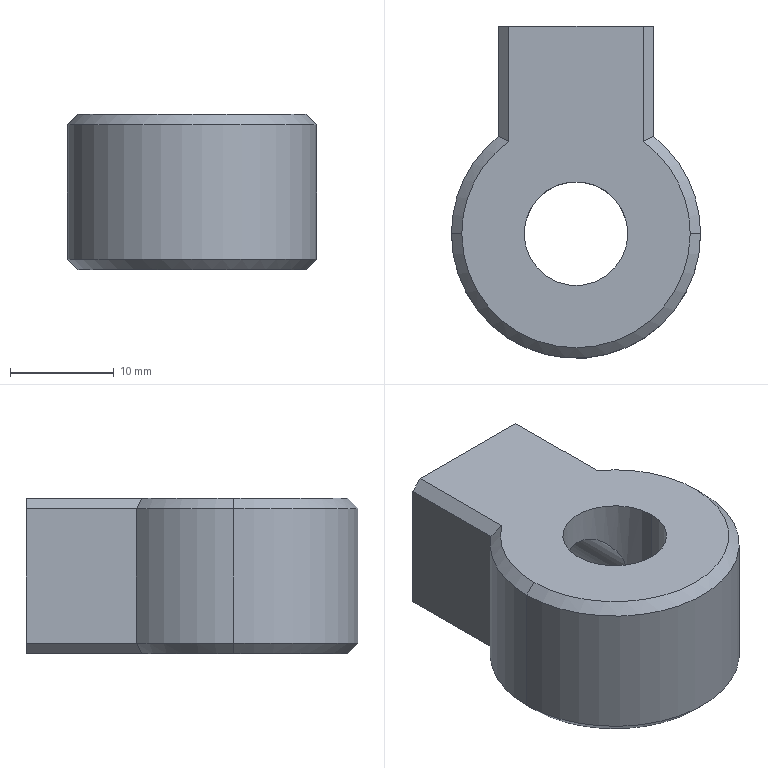Part | SolidWorks | features HoleWzd 2, Chamfer 1, Extrusion 1 | 1 solid | 22 faces | box 24 x 32 x 15 mm | volume 6636 mm3 | plane 9 | cylinder 7 | cone 6 | commonest cylinder face diameters 24 x3 8.5 x2 10 x2
STEP:
#1=CARTESIAN_POINT('',(11.,0.,7.5));
#2=VERTEX_POINT('',#1);
#3=CARTESIAN_POINT('',(6.5,8.874,7.5));
#4=VERTEX_POINT('',#3);
#5=CARTESIAN_POINT('',(0.,0.,7.5));
#6=DIRECTION('',(0.,0.,1.));
#7=DIRECTION('',(1.,0.,0.));
#8=AXIS2_PLACEMENT_3D('',#5,#6,#7);
#9=CIRCLE('',#8,11.);
#10=EDGE_CURVE('',#2,#4,#9,.T.);
#11=ORIENTED_EDGE('',*,*,#10,.F.);
#12=CARTESIAN_POINT('',(12.,0.,6.5));
#13=VERTEX_POINT('',#12);
#14=CARTESIAN_POINT('',(11.,0.,7.5));
#15=DIRECTION('',(0.7071,0.,-0.7071));
#16=VECTOR('',#15,1000.);
#17=LINE('',#14,#16);
#18=EDGE_CURVE('',#2,#13,#17,.T.);
#19=ORIENTED_EDGE('',*,*,#18,.T.);
#20=CARTESIAN_POINT('',(7.5,9.367,6.5));
#21=VERTEX_POINT('',#20);
#22=CARTESIAN_POINT('',(0.,0.,6.5));
#23=DIRECTION('',(0.,0.,-1.));
#24=DIRECTION('',(1.,0.,0.));
#25=AXIS2_PLACEMENT_3D('',#22,#23,#24);
#26=CIRCLE('',#25,12.);
#27=EDGE_CURVE('',#21,#13,#26,.T.);
#28=ORIENTED_EDGE('',*,*,#27,.F.);
#29=CARTESIAN_POINT('',(6.5,8.874,7.5));
#30=CARTESIAN_POINT('',(6.832,9.043,7.168));
#31=CARTESIAN_POINT('',(7.166,9.207,6.834));
#32=CARTESIAN_POINT('',(7.5,9.367,6.5));
#33=B_SPLINE_CURVE_WITH_KNOTS('',3,(#29,#30,#31,#32),.UNSPECIFIED.,.F.,.F.,(4,4),(0.,0.001498),.UNSPECIFIED.);
#34=EDGE_CURVE('',#4,#21,#33,.T.);
#35=ORIENTED_EDGE('',*,*,#34,.F.);
#36=EDGE_LOOP('',(#11,#19,#28,#35));
#37=FACE_OUTER_BOUND('',#36,.T.);
#38=CARTESIAN_POINT('',(0.,0.,7.5));
#39=DIRECTION('',(0.,0.,-1.));
#40=DIRECTION('',(-1.,0.,0.));
#41=AXIS2_PLACEMENT_3D('',#38,#39,#40);
#42=CONICAL_SURFACE('',#41,11.,0.7854);
#43=ADVANCED_FACE('',(#37),#42,.T.);
#44=ORIENTED_EDGE('',*,*,#18,.F.);
#45=CARTESIAN_POINT('',(-11.,0.,7.5));
#46=VERTEX_POINT('',#45);
#47=CARTESIAN_POINT('',(0.,0.,7.5));
#48=DIRECTION('',(0.,0.,1.));
#49=DIRECTION('',(1.,0.,0.));
#50=AXIS2_PLACEMENT_3D('',#47,#48,#49);
#51=CIRCLE('',#50,11.);
#52=EDGE_CURVE('',#46,#2,#51,.T.);
#53=ORIENTED_EDGE('',*,*,#52,.F.);
#54=CARTESIAN_POINT('',(-12.,0.,6.5));
#55=VERTEX_POINT('',#54);
#56=CARTESIAN_POINT('',(-11.,0.,7.5));
#57=DIRECTION('',(-0.7071,0.,-0.7071));
#58=VECTOR('',#57,1000.);
#59=LINE('',#56,#58);
#60=EDGE_CURVE('',#46,#55,#59,.T.);
#61=ORIENTED_EDGE('',*,*,#60,.T.);
#62=CARTESIAN_POINT('',(0.,0.,6.5));
#63=DIRECTION('',(0.,0.,-1.));
#64=DIRECTION('',(1.,0.,0.));
#65=AXIS2_PLACEMENT_3D('',#62,#63,#64);
#66=CIRCLE('',#65,12.);
#67=EDGE_CURVE('',#13,#55,#66,.T.);
#68=ORIENTED_EDGE('',*,*,#67,.F.);
#69=EDGE_LOOP('',(#44,#53,#61,#68));
#70=FACE_OUTER_BOUND('',#69,.T.);
#71=CARTESIAN_POINT('',(0.,0.,7.5));
#72=DIRECTION('',(0.,0.,-1.));
#73=DIRECTION('',(-1.,0.,0.));
#74=AXIS2_PLACEMENT_3D('',#71,#72,#73);
#75=CONICAL_SURFACE('',#74,11.,0.7854);
#76=ADVANCED_FACE('',(#70),#75,.T.);
#77=CARTESIAN_POINT('',(-11.,0.,-7.5));
#78=VERTEX_POINT('',#77);
#79=CARTESIAN_POINT('',(-6.5,8.874,-7.5));
#80=VERTEX_POINT('',#79);
#81=CARTESIAN_POINT('',(0.,0.,-7.5));
#82=DIRECTION('',(0.,0.,-1.));
#83=DIRECTION('',(1.,0.,0.));
#84=AXIS2_PLACEMENT_3D('',#81,#82,#83);
#85=CIRCLE('',#84,11.);
#86=EDGE_CURVE('',#78,#80,#85,.T.);
#87=ORIENTED_EDGE('',*,*,#86,.F.);
#88=CARTESIAN_POINT('',(-12.,0.,-6.5));
#89=VERTEX_POINT('',#88);
#90=CARTESIAN_POINT('',(-12.,0.,-6.5));
#91=DIRECTION('',(-0.7071,0.,0.7071));
#92=VECTOR('',#91,1000.);
#93=LINE('',#90,#92);
#94=EDGE_CURVE('',#78,#89,#93,.T.);
#95=ORIENTED_EDGE('',*,*,#94,.T.);
#96=CARTESIAN_POINT('',(-7.5,9.367,-6.5));
#97=VERTEX_POINT('',#96);
#98=CARTESIAN_POINT('',(0.,0.,-6.5));
#99=DIRECTION('',(0.,0.,1.));
#100=DIRECTION('',(1.,0.,0.));
#101=AXIS2_PLACEMENT_3D('',#98,#99,#100);
#102=CIRCLE('',#101,12.);
#103=EDGE_CURVE('',#97,#89,#102,.T.);
#104=ORIENTED_EDGE('',*,*,#103,.F.);
#105=CARTESIAN_POINT('',(-7.5,9.367,-6.5));
#106=CARTESIAN_POINT('',(-7.166,9.207,-6.834));
#107=CARTESIAN_POINT('',(-6.832,9.043,-7.168));
#108=CARTESIAN_POINT('',(-6.5,8.874,-7.5));
#109=B_SPLINE_CURVE_WITH_KNOTS('',3,(#105,#106,#107,#108),.UNSPECIFIED.,.F.,.F.,(4,4),(0.,0.001498),.UNSPECIFIED.);
#110=EDGE_CURVE('',#97,#80,#109,.T.);
#111=ORIENTED_EDGE('',*,*,#110,.T.);
#112=EDGE_LOOP('',(#87,#95,#104,#111));
#113=FACE_OUTER_BOUND('',#112,.T.);
#114=CARTESIAN_POINT('',(0.,0.,-6.5));
#115=DIRECTION('',(0.,0.,1.));
#116=DIRECTION('',(1.,0.,0.));
#117=AXIS2_PLACEMENT_3D('',#114,#115,#116);
#118=CONICAL_SURFACE('',#117,12.,0.7854);
#119=ADVANCED_FACE('',(#113),#118,.T.);
#120=ORIENTED_EDGE('',*,*,#94,.F.);
#121=CARTESIAN_POINT('',(11.,0.,-7.5));
#122=VERTEX_POINT('',#121);
#123=CARTESIAN_POINT('',(0.,0.,-7.5));
#124=DIRECTION('',(0.,0.,-1.));
#125=DIRECTION('',(1.,0.,0.));
#126=AXIS2_PLACEMENT_3D('',#123,#124,#125);
#127=CIRCLE('',#126,11.);
#128=EDGE_CURVE('',#122,#78,#127,.T.);
#129=ORIENTED_EDGE('',*,*,#128,.F.);
#130=CARTESIAN_POINT('',(12.,0.,-6.5));
#131=VERTEX_POINT('',#130);
#132=CARTESIAN_POINT('',(12.,0.,-6.5));
#133=DIRECTION('',(0.7071,0.,0.7071));
#134=VECTOR('',#133,1000.);
#135=LINE('',#132,#134);
#136=EDGE_CURVE('',#122,#131,#135,.T.);
#137=ORIENTED_EDGE('',*,*,#136,.T.);
#138=CARTESIAN_POINT('',(0.,0.,-6.5));
#139=DIRECTION('',(0.,0.,1.));
#140=DIRECTION('',(1.,0.,0.));
#141=AXIS2_PLACEMENT_3D('',#138,#139,#140);
#142=CIRCLE('',#141,12.);
#143=EDGE_CURVE('',#89,#131,#142,.T.);
#144=ORIENTED_EDGE('',*,*,#143,.F.);
#145=EDGE_LOOP('',(#120,#129,#137,#144));
#146=FACE_OUTER_BOUND('',#145,.T.);
#147=CARTESIAN_POINT('',(0.,0.,-6.5));
#148=DIRECTION('',(0.,0.,1.));
#149=DIRECTION('',(1.,0.,0.));
#150=AXIS2_PLACEMENT_3D('',#147,#148,#149);
#151=CONICAL_SURFACE('',#150,12.,0.7854);
#152=ADVANCED_FACE('',(#146),#151,.T.);
#153=CARTESIAN_POINT('',(0.,5.,-4.25));
#154=VERTEX_POINT('',#153);
#155=CARTESIAN_POINT('',(0.,5.,4.25));
#156=VERTEX_POINT('',#155);
#157=CARTESIAN_POINT('',(0.,5.,-4.25));
#158=CARTESIAN_POINT('',(-0.1486,5.,-4.25));
#159=CARTESIAN_POINT('',(-0.2969,4.993,-4.242));
#160=CARTESIAN_POINT('',(-0.5929,4.967,-4.211));
#161=CARTESIAN_POINT('',(-0.7415,4.947,-4.187));
#162=CARTESIAN_POINT('',(-1.174,4.869,-4.095));
#163=CARTESIAN_POINT('',(-1.449,4.794,-4.006));
#164=CARTESIAN_POINT('',(-1.973,4.603,-3.775));
#165=CARTESIAN_POINT('',(-2.212,4.491,-3.639));
#166=CARTESIAN_POINT('',(-2.656,4.244,-3.329));
#167=CARTESIAN_POINT('',(-2.861,4.107,-3.154));
#168=CARTESIAN_POINT('',(-3.228,3.826,-2.777));
#169=CARTESIAN_POINT('',(-3.39,3.681,-2.576));
#170=CARTESIAN_POINT('',(-3.679,3.392,-2.144));
#171=CARTESIAN_POINT('',(-3.805,3.248,-1.911));
#172=CARTESIAN_POINT('',(-4.016,2.984,-1.418));
#173=CARTESIAN_POINT('',(-4.1,2.864,-1.156));
#174=CARTESIAN_POINT('',(-4.189,2.731,-0.7336));
#175=CARTESIAN_POINT('',(-4.211,2.695,-0.5904));
#176=CARTESIAN_POINT('',(-4.242,2.647,-0.2976));
#177=CARTESIAN_POINT('',(-4.25,2.634,-0.1463));
#178=CARTESIAN_POINT('',(-4.25,2.634,0.1535));
#179=CARTESIAN_POINT('',(-4.242,2.647,0.3016));
#180=CARTESIAN_POINT('',(-4.211,2.696,0.5943));
#181=CARTESIAN_POINT('',(-4.188,2.733,0.74));
#182=CARTESIAN_POINT('',(-4.099,2.866,1.159));
#183=CARTESIAN_POINT('',(-4.015,2.985,1.419));
#184=CARTESIAN_POINT('',(-3.804,3.25,1.915));
#185=CARTESIAN_POINT('',(-3.678,3.393,2.144));
#186=CARTESIAN_POINT('',(-3.391,3.68,2.575));
#187=CARTESIAN_POINT('',(-3.228,3.826,2.777));
#188=CARTESIAN_POINT('',(-2.859,4.109,3.156));
#189=CARTESIAN_POINT('',(-2.656,4.244,3.329));
#190=CARTESIAN_POINT('',(-2.325,4.429,3.561));
#191=CARTESIAN_POINT('',(-2.209,4.487,3.633));
#192=CARTESIAN_POINT('',(-1.968,4.599,3.77));
#193=CARTESIAN_POINT('',(-1.841,4.651,3.833));
#194=CARTESIAN_POINT('',(-1.452,4.793,4.004));
#195=CARTESIAN_POINT('',(-1.178,4.868,4.094));
#196=CARTESIAN_POINT('',(-0.6,4.973,4.218));
#197=CARTESIAN_POINT('',(-0.3019,5.,4.25));
#198=CARTESIAN_POINT('',(0.,5.,4.25));
#199=B_SPLINE_CURVE_WITH_KNOTS('',3,(#157,#158,#159,#160,#161,#162,#163,#164,#165,#166,#167,#168,#169,#170,#171,#172,#173,#174,#175,#176,#177,#178,#179,#180,#181,#182,#183,#184,#185,#186,#187,#188,#189,#190,#191,#192,#193,#194,#195,#196,#197,#198),.UNSPECIFIED.,.F.,.F.,(4,2,2,2,2,2,2,2,2,2,2,2,2,2,2,2,2,2,2,2,4),(0.01424,0.01469,0.01513,0.01602,0.01692,0.01781,0.0187,0.01959,0.02048,0.02092,0.02137,0.02181,0.02226,0.02315,0.02404,0.02493,0.02582,0.02627,0.02671,0.0276,0.02849),.UNSPECIFIED.);
#200=EDGE_CURVE('',#154,#156,#199,.T.);
#201=ORIENTED_EDGE('',*,*,#200,.F.);
#202=CARTESIAN_POINT('',(0.,20.,-4.25));
#203=VERTEX_POINT('',#202);
#204=CARTESIAN_POINT('',(0.,20.,-4.25));
#205=DIRECTION('',(0.,1.,0.));
#206=VECTOR('',#205,1000.);
#207=LINE('',#204,#206);
#208=EDGE_CURVE('',#154,#203,#207,.T.);
#209=ORIENTED_EDGE('',*,*,#208,.T.);
#210=CARTESIAN_POINT('',(0.,20.,4.25));
#211=VERTEX_POINT('',#210);
#212=CARTESIAN_POINT('',(0.,20.,0.));
#213=DIRECTION('',(0.,1.,0.));
#214=DIRECTION('',(0.,0.,1.));
#215=AXIS2_PLACEMENT_3D('',#212,#213,#214);
#216=CIRCLE('',#215,4.25);
#217=EDGE_CURVE('',#203,#211,#216,.T.);
#218=ORIENTED_EDGE('',*,*,#217,.T.);
#219=CARTESIAN_POINT('',(0.,20.,4.25));
#220=DIRECTION('',(0.,1.,0.));
#221=VECTOR('',#220,1000.);
#222=LINE('',#219,#221);
#223=EDGE_CURVE('',#156,#211,#222,.T.);
#224=ORIENTED_EDGE('',*,*,#223,.F.);
#225=EDGE_LOOP('',(#201,#209,#218,#224));
#226=FACE_OUTER_BOUND('',#225,.T.);
#227=CARTESIAN_POINT('',(0.,20.,0.));
#228=DIRECTION('',(0.,1.,0.));
#229=DIRECTION('',(0.,0.,1.));
#230=AXIS2_PLACEMENT_3D('',#227,#228,#229);
#231=CYLINDRICAL_SURFACE('',#230,4.25);
#232=ADVANCED_FACE('',(#226),#231,.F.);
#233=CARTESIAN_POINT('',(-5.,0.,-7.5));
#234=VERTEX_POINT('',#233);
#235=CARTESIAN_POINT('',(5.,0.,-7.5));
#236=VERTEX_POINT('',#235);
#237=CARTESIAN_POINT('',(0.,0.,-7.5));
#238=DIRECTION('',(0.,0.,1.));
#239=DIRECTION('',(1.,0.,0.));
#240=AXIS2_PLACEMENT_3D('',#237,#238,#239);
#241=CIRCLE('',#240,5.);
#242=EDGE_CURVE('',#234,#236,#241,.T.);
#243=ORIENTED_EDGE('',*,*,#242,.F.);
#244=CARTESIAN_POINT('',(-5.,0.,7.5));
#245=VERTEX_POINT('',#244);
#246=CARTESIAN_POINT('',(-5.,0.,7.5));
#247=DIRECTION('',(0.,0.,1.));
#248=VECTOR('',#247,1000.);
#249=LINE('',#246,#248);
#250=EDGE_CURVE('',#234,#245,#249,.T.);
#251=ORIENTED_EDGE('',*,*,#250,.T.);
#252=CARTESIAN_POINT('',(5.,0.,7.5));
#253=VERTEX_POINT('',#252);
#254=CARTESIAN_POINT('',(0.,0.,7.5));
#255=DIRECTION('',(0.,0.,1.));
#256=DIRECTION('',(1.,0.,0.));
#257=AXIS2_PLACEMENT_3D('',#254,#255,#256);
#258=CIRCLE('',#257,5.);
#259=EDGE_CURVE('',#245,#253,#258,.T.);
#260=ORIENTED_EDGE('',*,*,#259,.T.);
#261=CARTESIAN_POINT('',(5.,0.,7.5));
#262=DIRECTION('',(0.,0.,1.));
#263=VECTOR('',#262,1000.);
#264=LINE('',#261,#263);
#265=EDGE_CURVE('',#236,#253,#264,.T.);
#266=ORIENTED_EDGE('',*,*,#265,.F.);
#267=EDGE_LOOP('',(#243,#251,#260,#266));
#268=FACE_OUTER_BOUND('',#267,.T.);
#269=CARTESIAN_POINT('',(0.,0.,7.5));
#270=DIRECTION('',(0.,0.,1.));
#271=DIRECTION('',(1.,0.,0.));
#272=AXIS2_PLACEMENT_3D('',#269,#270,#271);
#273=CYLINDRICAL_SURFACE('',#272,5.);
#274=ADVANCED_FACE('',(#268),#273,.F.);
#275=ORIENTED_EDGE('',*,*,#103,.T.);
#276=CARTESIAN_POINT('',(-12.,0.,-7.5));
#277=DIRECTION('',(0.,0.,1.));
#278=VECTOR('',#277,1000.);
#279=LINE('',#276,#278);
#280=EDGE_CURVE('',#89,#55,#279,.T.);
#281=ORIENTED_EDGE('',*,*,#280,.T.);
#282=CARTESIAN_POINT('',(-7.5,9.367,6.5));
#283=VERTEX_POINT('',#282);
#284=CARTESIAN_POINT('',(0.,0.,6.5));
#285=DIRECTION('',(0.,0.,-1.));
#286=DIRECTION('',(1.,0.,0.));
#287=AXIS2_PLACEMENT_3D('',#284,#285,#286);
#288=CIRCLE('',#287,12.);
#289=EDGE_CURVE('',#55,#283,#288,.T.);
#290=ORIENTED_EDGE('',*,*,#289,.T.);
#291=CARTESIAN_POINT('',(-7.5,9.367,-7.5));
#292=DIRECTION('',(0.,0.,1.));
#293=VECTOR('',#292,1000.);
#294=LINE('',#291,#293);
#295=EDGE_CURVE('',#97,#283,#294,.T.);
#296=ORIENTED_EDGE('',*,*,#295,.F.);
#297=EDGE_LOOP('',(#275,#281,#290,#296));
#298=FACE_OUTER_BOUND('',#297,.T.);
#299=CARTESIAN_POINT('',(0.,0.,-7.5));
#300=DIRECTION('',(0.,0.,1.));
#301=DIRECTION('',(1.,0.,0.));
#302=AXIS2_PLACEMENT_3D('',#299,#300,#301);
#303=CYLINDRICAL_SURFACE('',#302,12.);
#304=ADVANCED_FACE('',(#298),#303,.T.);
#305=ORIENTED_EDGE('',*,*,#280,.F.);
#306=ORIENTED_EDGE('',*,*,#143,.T.);
#307=CARTESIAN_POINT('',(12.,0.,-7.5));
#308=DIRECTION('',(0.,0.,1.));
#309=VECTOR('',#308,1000.);
#310=LINE('',#307,#309);
#311=EDGE_CURVE('',#131,#13,#310,.T.);
#312=ORIENTED_EDGE('',*,*,#311,.T.);
#313=ORIENTED_EDGE('',*,*,#67,.T.);
#314=EDGE_LOOP('',(#305,#306,#312,#313));
#315=FACE_OUTER_BOUND('',#314,.T.);
#316=CARTESIAN_POINT('',(0.,0.,-7.5));
#317=DIRECTION('',(0.,0.,1.));
#318=DIRECTION('',(1.,0.,0.));
#319=AXIS2_PLACEMENT_3D('',#316,#317,#318);
#320=CYLINDRICAL_SURFACE('',#319,12.);
#321=ADVANCED_FACE('',(#315),#320,.T.);
#322=CARTESIAN_POINT('',(7.5,9.367,-6.5));
#323=VERTEX_POINT('',#322);
#324=CARTESIAN_POINT('',(7.5,9.367,-7.5));
#325=DIRECTION('',(0.,0.,1.));
#326=VECTOR('',#325,1000.);
#327=LINE('',#324,#326);
#328=EDGE_CURVE('',#323,#21,#327,.T.);
#329=ORIENTED_EDGE('',*,*,#328,.F.);
#330=CARTESIAN_POINT('',(7.5,20.,-6.5));
#331=VERTEX_POINT('',#330);
#332=CARTESIAN_POINT('',(7.5,20.,-6.5));
#333=DIRECTION('',(0.,1.,0.));
#334=VECTOR('',#333,1000.);
#335=LINE('',#332,#334);
#336=EDGE_CURVE('',#323,#331,#335,.T.);
#337=ORIENTED_EDGE('',*,*,#336,.T.);
#338=CARTESIAN_POINT('',(7.5,20.,6.5));
#339=VERTEX_POINT('',#338);
#340=CARTESIAN_POINT('',(7.5,20.,-7.5));
#341=DIRECTION('',(0.,0.,1.));
#342=VECTOR('',#341,1000.);
#343=LINE('',#340,#342);
#344=EDGE_CURVE('',#331,#339,#343,.T.);
#345=ORIENTED_EDGE('',*,*,#344,.T.);
#346=CARTESIAN_POINT('',(7.5,9.367,6.5));
#347=DIRECTION('',(0.,-1.,0.));
#348=VECTOR('',#347,1000.);
#349=LINE('',#346,#348);
#350=EDGE_CURVE('',#339,#21,#349,.T.);
#351=ORIENTED_EDGE('',*,*,#350,.T.);
#352=EDGE_LOOP('',(#329,#337,#345,#351));
#353=FACE_OUTER_BOUND('',#352,.T.);
#354=CARTESIAN_POINT('',(7.5,9.367,-7.5));
#355=DIRECTION('',(1.,0.,0.));
#356=DIRECTION('',(0.,0.,-1.));
#357=AXIS2_PLACEMENT_3D('',#354,#355,#356);
#358=PLANE('',#357);
#359=ADVANCED_FACE('',(#353),#358,.T.);
#360=ORIENTED_EDGE('',*,*,#311,.F.);
#361=CARTESIAN_POINT('',(0.,0.,-6.5));
#362=DIRECTION('',(0.,0.,1.));
#363=DIRECTION('',(1.,0.,0.));
#364=AXIS2_PLACEMENT_3D('',#361,#362,#363);
#365=CIRCLE('',#364,12.);
#366=EDGE_CURVE('',#131,#323,#365,.T.);
#367=ORIENTED_EDGE('',*,*,#366,.T.);
#368=ORIENTED_EDGE('',*,*,#328,.T.);
#369=ORIENTED_EDGE('',*,*,#27,.T.);
#370=EDGE_LOOP('',(#360,#367,#368,#369));
#371=FACE_OUTER_BOUND('',#370,.T.);
#372=CARTESIAN_POINT('',(0.,0.,-7.5));
#373=DIRECTION('',(0.,0.,1.));
#374=DIRECTION('',(1.,0.,0.));
#375=AXIS2_PLACEMENT_3D('',#372,#373,#374);
#376=CYLINDRICAL_SURFACE('',#375,12.);
#377=ADVANCED_FACE('',(#371),#376,.T.);
#378=CARTESIAN_POINT('',(-7.5,20.,-6.5));
#379=VERTEX_POINT('',#378);
#380=CARTESIAN_POINT('',(-7.5,20.,6.5));
#381=VERTEX_POINT('',#380);
#382=CARTESIAN_POINT('',(-7.5,20.,-7.5));
#383=DIRECTION('',(0.,0.,1.));
#384=VECTOR('',#383,1000.);
#385=LINE('',#382,#384);
#386=EDGE_CURVE('',#379,#381,#385,.T.);
#387=ORIENTED_EDGE('',*,*,#386,.F.);
#388=CARTESIAN_POINT('',(-7.5,9.367,-6.5));
#389=DIRECTION('',(0.,-1.,0.));
#390=VECTOR('',#389,1000.);
#391=LINE('',#388,#390);
#392=EDGE_CURVE('',#379,#97,#391,.T.);
#393=ORIENTED_EDGE('',*,*,#392,.T.);
#394=ORIENTED_EDGE('',*,*,#295,.T.);
#395=CARTESIAN_POINT('',(-7.5,20.,6.5));
#396=DIRECTION('',(0.,1.,0.));
#397=VECTOR('',#396,1000.);
#398=LINE('',#395,#397);
#399=EDGE_CURVE('',#283,#381,#398,.T.);
#400=ORIENTED_EDGE('',*,*,#399,.T.);
#401=EDGE_LOOP('',(#387,#393,#394,#400));
#402=FACE_OUTER_BOUND('',#401,.T.);
#403=CARTESIAN_POINT('',(-7.5,20.,-7.5));
#404=DIRECTION('',(-1.,0.,0.));
#405=DIRECTION('',(0.,-1.,0.));
#406=AXIS2_PLACEMENT_3D('',#403,#404,#405);
#407=PLANE('',#406);
#408=ADVANCED_FACE('',(#402),#407,.T.);
#409=CARTESIAN_POINT('',(0.,20.,0.));
#410=DIRECTION('',(0.,1.,0.));
#411=DIRECTION('',(0.,0.,1.));
#412=AXIS2_PLACEMENT_3D('',#409,#410,#411);
#413=CIRCLE('',#412,4.25);
#414=EDGE_CURVE('',#211,#203,#413,.T.);
#415=ORIENTED_EDGE('',*,*,#414,.F.);
#416=ORIENTED_EDGE('',*,*,#217,.F.);
#417=EDGE_LOOP('',(#415,#416));
#418=FACE_BOUND('',#417,.T.);
#419=ORIENTED_EDGE('',*,*,#344,.F.);
#420=CARTESIAN_POINT('',(6.5,20.,-7.5));
#421=VERTEX_POINT('',#420);
#422=CARTESIAN_POINT('',(7.,20.,-7.));
#423=DIRECTION('',(-0.7071,0.,-0.7071));
#424=VECTOR('',#423,1000.);
#425=LINE('',#422,#424);
#426=EDGE_CURVE('',#331,#421,#425,.T.);
#427=ORIENTED_EDGE('',*,*,#426,.T.);
#428=CARTESIAN_POINT('',(-6.5,20.,-7.5));
#429=VERTEX_POINT('',#428);
#430=CARTESIAN_POINT('',(7.5,20.,-7.5));
#431=DIRECTION('',(-1.,0.,0.));
#432=VECTOR('',#431,1000.);
#433=LINE('',#430,#432);
#434=EDGE_CURVE('',#421,#429,#433,.T.);
#435=ORIENTED_EDGE('',*,*,#434,.T.);
#436=CARTESIAN_POINT('',(0.5,20.,-14.5));
#437=DIRECTION('',(-0.7071,0.,0.7071));
#438=VECTOR('',#437,1000.);
#439=LINE('',#436,#438);
#440=EDGE_CURVE('',#429,#379,#439,.T.);
#441=ORIENTED_EDGE('',*,*,#440,.T.);
#442=ORIENTED_EDGE('',*,*,#386,.T.);
#443=CARTESIAN_POINT('',(-6.5,20.,7.5));
#444=VERTEX_POINT('',#443);
#445=CARTESIAN_POINT('',(-7.,20.,7.));
#446=DIRECTION('',(0.7071,0.,0.7071));
#447=VECTOR('',#446,1000.);
#448=LINE('',#445,#447);
#449=EDGE_CURVE('',#381,#444,#448,.T.);
#450=ORIENTED_EDGE('',*,*,#449,.T.);
#451=CARTESIAN_POINT('',(6.5,20.,7.5));
#452=VERTEX_POINT('',#451);
#453=CARTESIAN_POINT('',(7.5,20.,7.5));
#454=DIRECTION('',(-1.,0.,0.));
#455=VECTOR('',#454,1000.);
#456=LINE('',#453,#455);
#457=EDGE_CURVE('',#452,#444,#456,.T.);
#458=ORIENTED_EDGE('',*,*,#457,.F.);
#459=CARTESIAN_POINT('',(14.5,20.,-0.5));
#460=DIRECTION('',(0.7071,0.,-0.7071));
#461=VECTOR('',#460,1000.);
#462=LINE('',#459,#461);
#463=EDGE_CURVE('',#452,#339,#462,.T.);
#464=ORIENTED_EDGE('',*,*,#463,.T.);
#465=EDGE_LOOP('',(#419,#427,#435,#441,#442,#450,#458,#464));
#466=FACE_OUTER_BOUND('',#465,.T.);
#467=CARTESIAN_POINT('',(7.5,20.,-7.5));
#468=DIRECTION('',(0.,1.,0.));
#469=DIRECTION('',(0.,0.,1.));
#470=AXIS2_PLACEMENT_3D('',#467,#468,#469);
#471=PLANE('',#470);
#472=ADVANCED_FACE('',(#418,#466),#471,.T.);
#473=CARTESIAN_POINT('',(0.,0.,-7.5));
#474=DIRECTION('',(0.,0.,1.));
#475=DIRECTION('',(1.,0.,0.));
#476=AXIS2_PLACEMENT_3D('',#473,#474,#475);
#477=CIRCLE('',#476,5.);
#478=EDGE_CURVE('',#236,#234,#477,.T.);
#479=ORIENTED_EDGE('',*,*,#478,.T.);
#480=ORIENTED_EDGE('',*,*,#242,.T.);
#481=EDGE_LOOP('',(#479,#480));
#482=FACE_BOUND('',#481,.T.);
#483=ORIENTED_EDGE('',*,*,#434,.F.);
#484=CARTESIAN_POINT('',(6.5,8.874,-7.5));
#485=VERTEX_POINT('',#484);
#486=CARTESIAN_POINT('',(6.5,9.367,-7.5));
#487=DIRECTION('',(0.,-1.,0.));
#488=VECTOR('',#487,1000.);
#489=LINE('',#486,#488);
#490=EDGE_CURVE('',#421,#485,#489,.T.);
#491=ORIENTED_EDGE('',*,*,#490,.T.);
#492=CARTESIAN_POINT('',(0.,0.,-7.5));
#493=DIRECTION('',(0.,0.,-1.));
#494=DIRECTION('',(1.,0.,0.));
#495=AXIS2_PLACEMENT_3D('',#492,#493,#494);
#496=CIRCLE('',#495,11.);
#497=EDGE_CURVE('',#485,#122,#496,.T.);
#498=ORIENTED_EDGE('',*,*,#497,.T.);
#499=ORIENTED_EDGE('',*,*,#128,.T.);
#500=ORIENTED_EDGE('',*,*,#86,.T.);
#501=CARTESIAN_POINT('',(-6.5,20.,-7.5));
#502=DIRECTION('',(0.,1.,0.));
#503=VECTOR('',#502,1000.);
#504=LINE('',#501,#503);
#505=EDGE_CURVE('',#80,#429,#504,.T.);
#506=ORIENTED_EDGE('',*,*,#505,.T.);
#507=EDGE_LOOP('',(#483,#491,#498,#499,#500,#506));
#508=FACE_OUTER_BOUND('',#507,.T.);
#509=CARTESIAN_POINT('',(0.,0.,-7.5));
#510=DIRECTION('',(0.,0.,1.));
#511=DIRECTION('',(1.,0.,0.));
#512=AXIS2_PLACEMENT_3D('',#509,#510,#511);
#513=PLANE('',#512);
#514=ADVANCED_FACE('',(#482,#508),#513,.F.);
#515=CARTESIAN_POINT('',(0.,0.,7.5));
#516=DIRECTION('',(0.,0.,1.));
#517=DIRECTION('',(1.,0.,0.));
#518=AXIS2_PLACEMENT_3D('',#515,#516,#517);
#519=CIRCLE('',#518,5.);
#520=EDGE_CURVE('',#253,#245,#519,.T.);
#521=ORIENTED_EDGE('',*,*,#520,.F.);
#522=ORIENTED_EDGE('',*,*,#259,.F.);
#523=EDGE_LOOP('',(#521,#522));
#524=FACE_BOUND('',#523,.T.);
#525=CARTESIAN_POINT('',(-6.5,8.874,7.5));
#526=VERTEX_POINT('',#525);
#527=CARTESIAN_POINT('',(0.,0.,7.5));
#528=DIRECTION('',(0.,0.,1.));
#529=DIRECTION('',(1.,0.,0.));
#530=AXIS2_PLACEMENT_3D('',#527,#528,#529);
#531=CIRCLE('',#530,11.);
#532=EDGE_CURVE('',#526,#46,#531,.T.);
#533=ORIENTED_EDGE('',*,*,#532,.T.);
#534=ORIENTED_EDGE('',*,*,#52,.T.);
#535=ORIENTED_EDGE('',*,*,#10,.T.);
#536=CARTESIAN_POINT('',(6.5,0.,7.5));
#537=DIRECTION('',(0.,1.,0.));
#538=VECTOR('',#537,1000.);
#539=LINE('',#536,#538);
#540=EDGE_CURVE('',#4,#452,#539,.T.);
#541=ORIENTED_EDGE('',*,*,#540,.T.);
#542=ORIENTED_EDGE('',*,*,#457,.T.);
#543=CARTESIAN_POINT('',(-6.5,0.,7.5));
#544=DIRECTION('',(0.,-1.,0.));
#545=VECTOR('',#544,1000.);
#546=LINE('',#543,#545);
#547=EDGE_CURVE('',#444,#526,#546,.T.);
#548=ORIENTED_EDGE('',*,*,#547,.T.);
#549=EDGE_LOOP('',(#533,#534,#535,#541,#542,#548));
#550=FACE_OUTER_BOUND('',#549,.T.);
#551=CARTESIAN_POINT('',(0.,0.,7.5));
#552=DIRECTION('',(0.,0.,1.));
#553=DIRECTION('',(1.,0.,0.));
#554=AXIS2_PLACEMENT_3D('',#551,#552,#553);
#555=PLANE('',#554);
#556=ADVANCED_FACE('',(#524,#550),#555,.T.);
#557=ORIENTED_EDGE('',*,*,#250,.F.);
#558=ORIENTED_EDGE('',*,*,#478,.F.);
#559=ORIENTED_EDGE('',*,*,#265,.T.);
#560=ORIENTED_EDGE('',*,*,#520,.T.);
#561=EDGE_LOOP('',(#557,#558,#559,#560));
#562=FACE_OUTER_BOUND('',#561,.T.);
#563=CARTESIAN_POINT('',(0.,5.,4.25));
#564=CARTESIAN_POINT('',(0.3018,5.,4.25));
#565=CARTESIAN_POINT('',(0.5958,4.973,4.218));
#566=CARTESIAN_POINT('',(1.026,4.896,4.127));
#567=CARTESIAN_POINT('',(1.169,4.864,4.089));
#568=CARTESIAN_POINT('',(1.445,4.789,3.999));
#569=CARTESIAN_POINT('',(1.579,4.746,3.948));
#570=CARTESIAN_POINT('',(1.967,4.605,3.778));
#571=CARTESIAN_POINT('',(2.211,4.492,3.64));
#572=CARTESIAN_POINT('',(2.656,4.244,3.329));
#573=CARTESIAN_POINT('',(2.857,4.11,3.157));
#574=CARTESIAN_POINT('',(3.223,3.829,2.782));
#575=CARTESIAN_POINT('',(3.389,3.682,2.577));
#576=CARTESIAN_POINT('',(3.679,3.393,2.144));
#577=CARTESIAN_POINT('',(3.803,3.25,1.916));
#578=CARTESIAN_POINT('',(4.013,2.987,1.424));
#579=CARTESIAN_POINT('',(4.099,2.866,1.159));
#580=CARTESIAN_POINT('',(4.187,2.733,0.7408));
#581=CARTESIAN_POINT('',(4.211,2.697,0.5959));
#582=CARTESIAN_POINT('',(4.242,2.647,0.3012));
#583=CARTESIAN_POINT('',(4.25,2.634,0.1534));
#584=CARTESIAN_POINT('',(4.25,2.634,-0.1432));
#585=CARTESIAN_POINT('',(4.242,2.646,-0.2932));
#586=CARTESIAN_POINT('',(4.212,2.695,-0.5889));
#587=CARTESIAN_POINT('',(4.189,2.731,-0.7324));
#588=CARTESIAN_POINT('',(4.13,2.819,-1.013));
#589=CARTESIAN_POINT('',(4.094,2.872,-1.15));
#590=CARTESIAN_POINT('',(4.01,2.987,-1.413));
#591=CARTESIAN_POINT('',(3.963,3.049,-1.54));
#592=CARTESIAN_POINT('',(3.807,3.246,-1.909));
#593=CARTESIAN_POINT('',(3.681,3.39,-2.14));
#594=CARTESIAN_POINT('',(3.39,3.681,-2.576));
#595=CARTESIAN_POINT('',(3.227,3.826,-2.778));
#596=CARTESIAN_POINT('',(2.86,4.107,-3.154));
#597=CARTESIAN_POINT('',(2.655,4.244,-3.33));
#598=CARTESIAN_POINT('',(2.211,4.492,-3.64));
#599=CARTESIAN_POINT('',(1.971,4.603,-3.776));
#600=CARTESIAN_POINT('',(1.45,4.793,-4.005));
#601=CARTESIAN_POINT('',(1.173,4.869,-4.095));
#602=CARTESIAN_POINT('',(0.5994,4.972,-4.218));
#603=CARTESIAN_POINT('',(0.2971,5.,-4.25));
#604=CARTESIAN_POINT('',(0.,5.,-4.25));
#605=B_SPLINE_CURVE_WITH_KNOTS('',3,(#563,#564,#565,#566,#567,#568,#569,#570,#571,#572,#573,#574,#575,#576,#577,#578,#579,#580,#581,#582,#583,#584,#585,#586,#587,#588,#589,#590,#591,#592,#593,#594,#595,#596,#597,#598,#599,#600,#601,#602,#603,#604),.UNSPECIFIED.,.F.,.F.,(4,2,2,2,2,2,2,2,2,2,2,2,2,2,2,2,2,2,2,2,4),(0.,0.0008902,0.001335,0.00178,0.002671,0.003561,0.004451,0.005341,0.006232,0.006677,0.007122,0.007567,0.008012,0.008457,0.008902,0.009792,0.01068,0.01157,0.01246,0.01335,0.01424),.UNSPECIFIED.);
#606=EDGE_CURVE('',#156,#154,#605,.T.);
#607=ORIENTED_EDGE('',*,*,#606,.T.);
#608=ORIENTED_EDGE('',*,*,#200,.T.);
#609=EDGE_LOOP('',(#607,#608));
#610=FACE_BOUND('',#609,.T.);
#611=CARTESIAN_POINT('',(0.,0.,7.5));
#612=DIRECTION('',(0.,0.,1.));
#613=DIRECTION('',(1.,0.,0.));
#614=AXIS2_PLACEMENT_3D('',#611,#612,#613);
#615=CYLINDRICAL_SURFACE('',#614,5.);
#616=ADVANCED_FACE('',(#562,#610),#615,.F.);
#617=ORIENTED_EDGE('',*,*,#208,.F.);
#618=ORIENTED_EDGE('',*,*,#606,.F.);
#619=ORIENTED_EDGE('',*,*,#223,.T.);
#620=ORIENTED_EDGE('',*,*,#414,.T.);
#621=EDGE_LOOP('',(#617,#618,#619,#620));
#622=FACE_OUTER_BOUND('',#621,.T.);
#623=CARTESIAN_POINT('',(0.,20.,0.));
#624=DIRECTION('',(0.,1.,0.));
#625=DIRECTION('',(0.,0.,1.));
#626=AXIS2_PLACEMENT_3D('',#623,#624,#625);
#627=CYLINDRICAL_SURFACE('',#626,4.25);
#628=ADVANCED_FACE('',(#622),#627,.F.);
#629=ORIENTED_EDGE('',*,*,#440,.F.);
#630=ORIENTED_EDGE('',*,*,#505,.F.);
#631=ORIENTED_EDGE('',*,*,#110,.F.);
#632=ORIENTED_EDGE('',*,*,#392,.F.);
#633=EDGE_LOOP('',(#629,#630,#631,#632));
#634=FACE_OUTER_BOUND('',#633,.T.);
#635=CARTESIAN_POINT('',(-7.5,20.,-6.5));
#636=DIRECTION('',(-0.7071,0.,-0.7071));
#637=DIRECTION('',(0.,1.,0.));
#638=AXIS2_PLACEMENT_3D('',#635,#636,#637);
#639=PLANE('',#638);
#640=ADVANCED_FACE('',(#634),#639,.T.);
#641=ORIENTED_EDGE('',*,*,#136,.F.);
#642=ORIENTED_EDGE('',*,*,#497,.F.);
#643=CARTESIAN_POINT('',(7.5,9.367,-6.5));
#644=CARTESIAN_POINT('',(7.166,9.207,-6.834));
#645=CARTESIAN_POINT('',(6.832,9.043,-7.168));
#646=CARTESIAN_POINT('',(6.5,8.874,-7.5));
#647=B_SPLINE_CURVE_WITH_KNOTS('',3,(#643,#644,#645,#646),.UNSPECIFIED.,.F.,.F.,(4,4),(0.,0.001498),.UNSPECIFIED.);
#648=EDGE_CURVE('',#323,#485,#647,.T.);
#649=ORIENTED_EDGE('',*,*,#648,.F.);
#650=ORIENTED_EDGE('',*,*,#366,.F.);
#651=EDGE_LOOP('',(#641,#642,#649,#650));
#652=FACE_OUTER_BOUND('',#651,.T.);
#653=CARTESIAN_POINT('',(0.,0.,-6.5));
#654=DIRECTION('',(0.,0.,1.));
#655=DIRECTION('',(1.,0.,0.));
#656=AXIS2_PLACEMENT_3D('',#653,#654,#655);
#657=CONICAL_SURFACE('',#656,12.,0.7854);
#658=ADVANCED_FACE('',(#652),#657,.T.);
#659=ORIENTED_EDGE('',*,*,#648,.T.);
#660=ORIENTED_EDGE('',*,*,#490,.F.);
#661=ORIENTED_EDGE('',*,*,#426,.F.);
#662=ORIENTED_EDGE('',*,*,#336,.F.);
#663=EDGE_LOOP('',(#659,#660,#661,#662));
#664=FACE_OUTER_BOUND('',#663,.T.);
#665=CARTESIAN_POINT('',(7.5,9.367,-6.5));
#666=DIRECTION('',(0.7071,0.,-0.7071));
#667=DIRECTION('',(0.,-1.,0.));
#668=AXIS2_PLACEMENT_3D('',#665,#666,#667);
#669=PLANE('',#668);
#670=ADVANCED_FACE('',(#664),#669,.T.);
#671=ORIENTED_EDGE('',*,*,#449,.F.);
#672=ORIENTED_EDGE('',*,*,#399,.F.);
#673=CARTESIAN_POINT('',(-6.5,8.874,7.5));
#674=CARTESIAN_POINT('',(-6.832,9.043,7.168));
#675=CARTESIAN_POINT('',(-7.166,9.207,6.834));
#676=CARTESIAN_POINT('',(-7.5,9.367,6.5));
#677=B_SPLINE_CURVE_WITH_KNOTS('',3,(#673,#674,#675,#676),.UNSPECIFIED.,.F.,.F.,(4,4),(0.,0.001498),.UNSPECIFIED.);
#678=EDGE_CURVE('',#526,#283,#677,.T.);
#679=ORIENTED_EDGE('',*,*,#678,.F.);
#680=ORIENTED_EDGE('',*,*,#547,.F.);
#681=EDGE_LOOP('',(#671,#672,#679,#680));
#682=FACE_OUTER_BOUND('',#681,.T.);
#683=CARTESIAN_POINT('',(-6.5,0.,7.5));
#684=DIRECTION('',(0.7071,0.,-0.7071));
#685=DIRECTION('',(0.,-1.,0.));
#686=AXIS2_PLACEMENT_3D('',#683,#684,#685);
#687=PLANE('',#686);
#688=ADVANCED_FACE('',(#682),#687,.F.);
#689=ORIENTED_EDGE('',*,*,#60,.F.);
#690=ORIENTED_EDGE('',*,*,#532,.F.);
#691=ORIENTED_EDGE('',*,*,#678,.T.);
#692=ORIENTED_EDGE('',*,*,#289,.F.);
#693=EDGE_LOOP('',(#689,#690,#691,#692));
#694=FACE_OUTER_BOUND('',#693,.T.);
#695=CARTESIAN_POINT('',(0.,0.,7.5));
#696=DIRECTION('',(0.,0.,-1.));
#697=DIRECTION('',(-1.,0.,0.));
#698=AXIS2_PLACEMENT_3D('',#695,#696,#697);
#699=CONICAL_SURFACE('',#698,11.,0.7854);
#700=ADVANCED_FACE('',(#694),#699,.T.);
#701=ORIENTED_EDGE('',*,*,#34,.T.);
#702=ORIENTED_EDGE('',*,*,#350,.F.);
#703=ORIENTED_EDGE('',*,*,#463,.F.);
#704=ORIENTED_EDGE('',*,*,#540,.F.);
#705=EDGE_LOOP('',(#701,#702,#703,#704));
#706=FACE_OUTER_BOUND('',#705,.T.);
#707=CARTESIAN_POINT('',(6.5,0.,7.5));
#708=DIRECTION('',(-0.7071,0.,-0.7071));
#709=DIRECTION('',(0.,1.,0.));
#710=AXIS2_PLACEMENT_3D('',#707,#708,#709);
#711=PLANE('',#710);
#712=ADVANCED_FACE('',(#706),#711,.F.);
#713=CLOSED_SHELL('',(#43,#76,#119,#152,#232,#274,#304,#321,#359,#377,#408,#472,#514,#556,#616,#628,#640,#658,#670,#688,#700,#712));
#714=MANIFOLD_SOLID_BREP('',#713);
#715=CARTESIAN_POINT('',(0.,0.,0.));
#716=DIRECTION('',(0.,0.,1.));
#717=DIRECTION('',(1.,0.,0.));
#718=AXIS2_PLACEMENT_3D('',#715,#716,#717);
#719=(LENGTH_UNIT()NAMED_UNIT(*)SI_UNIT(.MILLI.,.METRE.));
#720=UNCERTAINTY_MEASURE_WITH_UNIT(LENGTH_MEASURE(0.00001),#719,'','');
#721=(NAMED_UNIT(*)PLANE_ANGLE_UNIT()SI_UNIT($,.RADIAN.));
#722=(NAMED_UNIT(*)SI_UNIT($,.STERADIAN.)SOLID_ANGLE_UNIT());
#723=(GEOMETRIC_REPRESENTATION_CONTEXT(3)GLOBAL_UNCERTAINTY_ASSIGNED_CONTEXT((#720))GLOBAL_UNIT_ASSIGNED_CONTEXT((#719,#721,#722))REPRESENTATION_CONTEXT('',''));
#724=ADVANCED_BREP_SHAPE_REPRESENTATION('',(#714,#718),#723);